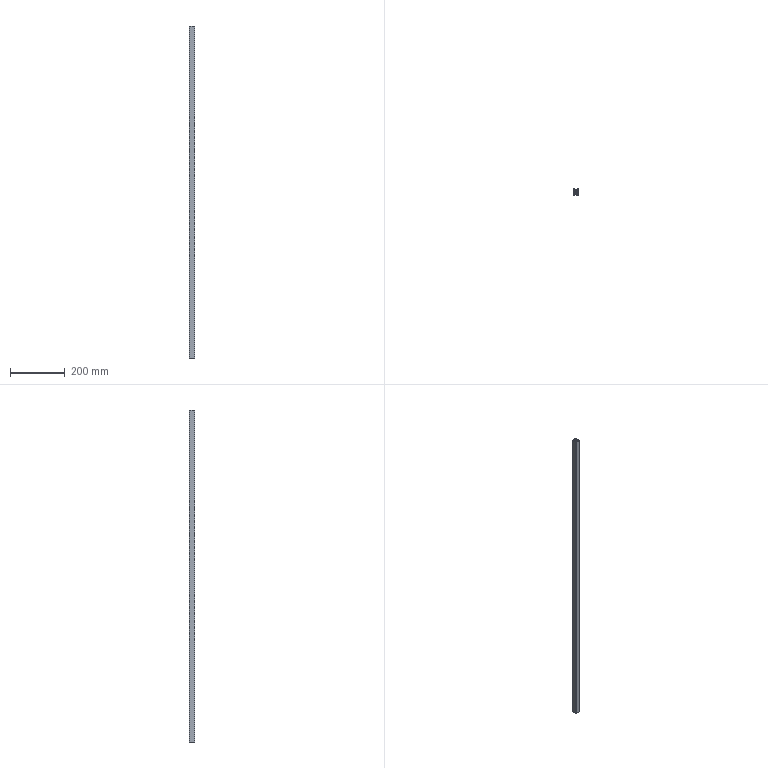Part | SolidWorks | features Extrusion 1 | 1 solid | 72 faces | box 20 x 20 x 1215 mm | volume 239025 mm3 | plane 38 | cylinder 34 | commonest cylinder face diameters 0.6 x20 4 x8 3 x4 5 x2